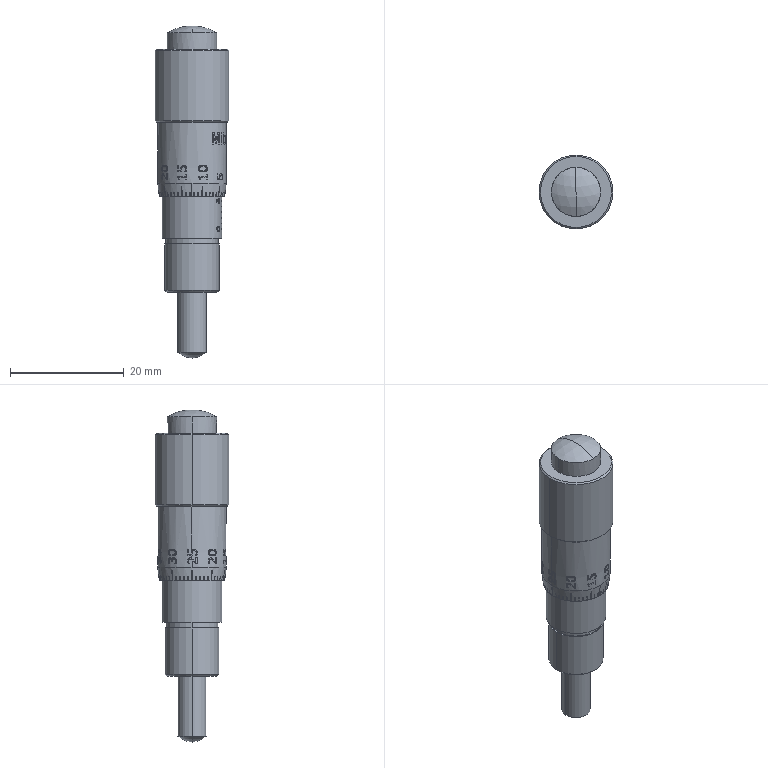Part | STEP file | 2 solids | 826 faces | box 13 x 13 x 58.395 mm | volume 4313 mm3 | plane 388 | spline 257 | cylinder 116 | cone 61 | torus 2 | sphere 2 | commonest cylinder face diameters 11.684 x40 12.014 x29 11.938 x11 12.065 x11 10.427 x6 10.478 x3